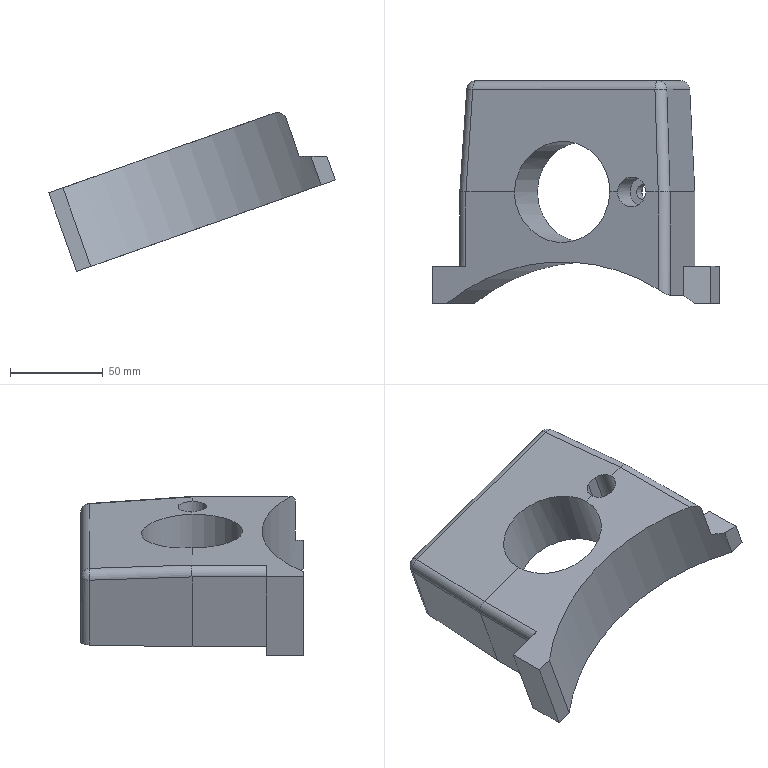Part | STEP file | SLIDE1-1_id622_x_t | 1 solid | 34 faces | box 154.532 x 120 x 85.769 mm | volume 429679 mm3 | plane 19 | cylinder 13 | other 2 | commonest cylinder face diameters 10 x7 8.5 x1 14 x1 16 x1 54.5 x1 71 x1
STEP:
#1=CARTESIAN_POINT('',(40.369,7.5,-42.76));
#2=VERTEX_POINT('',#1);
#3=CARTESIAN_POINT('',(35.121,7.5,-44.618));
#4=VERTEX_POINT('',#3);
#5=CARTESIAN_POINT('',(17.953,7.5,-50.698));
#6=DIRECTION('',(-0.9426,0.,-0.3338));
#7=VECTOR('',#6,1.);
#8=LINE('',#5,#7);
#9=EDGE_CURVE('',#2,#4,#8,.T.);
#10=ORIENTED_EDGE('',*,*,#9,.F.);
#11=CARTESIAN_POINT('',(33.824,7.5,-24.277));
#12=VERTEX_POINT('',#11);
#13=CARTESIAN_POINT('',(33.693,7.5,-23.907));
#14=DIRECTION('',(-0.3338,0.,0.9426));
#15=VECTOR('',#14,1.);
#16=LINE('',#13,#15);
#17=EDGE_CURVE('',#2,#12,#16,.T.);
#18=ORIENTED_EDGE('',*,*,#17,.T.);
#19=CARTESIAN_POINT('',(28.576,7.5,-26.136));
#20=VERTEX_POINT('',#19);
#21=CARTESIAN_POINT('',(-62.86,7.5,-58.515));
#22=DIRECTION('',(-0.9426,0.,-0.3338));
#23=VECTOR('',#22,1.);
#24=LINE('',#21,#23);
#25=EDGE_CURVE('',#12,#20,#24,.T.);
#26=ORIENTED_EDGE('',*,*,#25,.T.);
#27=CARTESIAN_POINT('',(28.444,7.5,-25.765));
#28=DIRECTION('',(0.3338,0.,-0.9426));
#29=VECTOR('',#28,1.);
#30=LINE('',#27,#29);
#31=EDGE_CURVE('',#20,#4,#30,.T.);
#32=ORIENTED_EDGE('',*,*,#31,.T.);
#33=EDGE_LOOP('',(#10,#18,#26,#32));
#34=FACE_OUTER_BOUND('',#33,.T.);
#35=CARTESIAN_POINT('',(33.693,7.5,-23.907));
#36=DIRECTION('',(0.,1.,0.));
#37=DIRECTION('',(0.,0.,1.));
#38=AXIS2_PLACEMENT_3D('',#35,#36,#37);
#39=PLANE('',#38);
#40=ADVANCED_FACE('',(#34),#39,.F.);
#41=CARTESIAN_POINT('',(41.751,0.,-42.27));
#42=VERTEX_POINT('',#41);
#43=CARTESIAN_POINT('',(33.739,0.,-45.108));
#44=VERTEX_POINT('',#43);
#45=CARTESIAN_POINT('',(41.751,0.,-42.27));
#46=CARTESIAN_POINT('',(41.751,-0.5406,-42.27));
#47=CARTESIAN_POINT('',(41.669,-1.031,-42.299));
#48=CARTESIAN_POINT('',(41.271,-2.098,-42.44));
#49=CARTESIAN_POINT('',(40.968,-2.591,-42.547));
#50=CARTESIAN_POINT('',(40.187,-3.42,-42.824));
#51=CARTESIAN_POINT('',(39.693,-3.753,-42.999));
#52=CARTESIAN_POINT('',(38.746,-4.15,-43.334));
#53=CARTESIAN_POINT('',(38.254,-4.25,-43.509));
#54=CARTESIAN_POINT('',(37.236,-4.25,-43.869));
#55=CARTESIAN_POINT('',(36.773,-4.163,-44.033));
#56=CARTESIAN_POINT('',(35.767,-3.74,-44.389));
#57=CARTESIAN_POINT('',(35.303,-3.42,-44.554));
#58=CARTESIAN_POINT('',(34.521,-2.591,-44.83));
#59=CARTESIAN_POINT('',(34.207,-2.066,-44.942));
#60=CARTESIAN_POINT('',(33.832,-1.062,-45.074));
#61=CARTESIAN_POINT('',(33.739,-0.541,-45.108));
#62=CARTESIAN_POINT('',(33.739,0.,-45.108));
#63=B_SPLINE_CURVE_WITH_KNOTS('',3,(#45,#46,#47,#48,#49,#50,#51,#52,#53,#54,#55,#56,#57,#58,#59,#60,#61,#62),.UNSPECIFIED.,.F.,.F.,(4,2,2,2,2,2,2,2,4),(0.,0.125,0.25,0.375,0.5,0.625,0.75,0.875,1.),.UNSPECIFIED.);
#64=EDGE_CURVE('',#42,#44,#63,.T.);
#65=ORIENTED_EDGE('',*,*,#64,.T.);
#66=CARTESIAN_POINT('',(33.739,0.,-45.108));
#67=CARTESIAN_POINT('',(33.739,0.5406,-45.108));
#68=CARTESIAN_POINT('',(33.821,1.031,-45.079));
#69=CARTESIAN_POINT('',(34.219,2.098,-44.938));
#70=CARTESIAN_POINT('',(34.521,2.591,-44.83));
#71=CARTESIAN_POINT('',(35.303,3.42,-44.554));
#72=CARTESIAN_POINT('',(35.797,3.753,-44.379));
#73=CARTESIAN_POINT('',(36.743,4.15,-44.044));
#74=CARTESIAN_POINT('',(37.236,4.25,-43.869));
#75=CARTESIAN_POINT('',(38.254,4.25,-43.509));
#76=CARTESIAN_POINT('',(38.717,4.163,-43.345));
#77=CARTESIAN_POINT('',(39.722,3.74,-42.989));
#78=CARTESIAN_POINT('',(40.187,3.42,-42.824));
#79=CARTESIAN_POINT('',(40.968,2.591,-42.547));
#80=CARTESIAN_POINT('',(41.282,2.066,-42.436));
#81=CARTESIAN_POINT('',(41.657,1.062,-42.304));
#82=CARTESIAN_POINT('',(41.751,0.541,-42.27));
#83=CARTESIAN_POINT('',(41.751,0.,-42.27));
#84=B_SPLINE_CURVE_WITH_KNOTS('',3,(#66,#67,#68,#69,#70,#71,#72,#73,#74,#75,#76,#77,#78,#79,#80,#81,#82,#83),.UNSPECIFIED.,.F.,.F.,(4,2,2,2,2,2,2,2,4),(0.,0.125,0.25,0.375,0.5,0.625,0.75,0.875,1.),.UNSPECIFIED.);
#85=EDGE_CURVE('',#44,#42,#84,.T.);
#86=ORIENTED_EDGE('',*,*,#85,.T.);
#87=EDGE_LOOP('',(#65,#86));
#88=FACE_BOUND('',#87,.T.);
#89=ORIENTED_EDGE('',*,*,#9,.T.);
#90=CARTESIAN_POINT('',(35.121,7.5,-44.618));
#91=CARTESIAN_POINT('',(34.318,7.184,-44.903));
#92=CARTESIAN_POINT('',(33.619,6.764,-45.15));
#93=CARTESIAN_POINT('',(32.238,5.548,-45.639));
#94=CARTESIAN_POINT('',(31.648,4.807,-45.848));
#95=CARTESIAN_POINT('',(30.744,3.127,-46.168));
#96=CARTESIAN_POINT('',(30.438,2.182,-46.276));
#97=CARTESIAN_POINT('',(30.161,0.3618,-46.374));
#98=CARTESIAN_POINT('',(30.176,-0.5477,-46.369));
#99=CARTESIAN_POINT('',(30.469,-2.281,-46.265));
#100=CARTESIAN_POINT('',(30.74,-3.113,-46.169));
#101=CARTESIAN_POINT('',(31.624,-4.769,-45.856));
#102=CARTESIAN_POINT('',(32.207,-5.516,-45.65));
#103=CARTESIAN_POINT('',(33.606,-6.757,-45.155));
#104=CARTESIAN_POINT('',(34.429,-7.244,-44.863));
#105=CARTESIAN_POINT('',(36.069,-7.854,-44.283));
#106=CARTESIAN_POINT('',(36.915,-8.,-43.983));
#107=CARTESIAN_POINT('',(38.575,-8.,-43.395));
#108=CARTESIAN_POINT('',(39.394,-7.864,-43.105));
#109=CARTESIAN_POINT('',(41.088,-7.234,-42.505));
#110=CARTESIAN_POINT('',(41.883,-6.757,-42.223));
#111=CARTESIAN_POINT('',(43.283,-5.516,-41.728));
#112=CARTESIAN_POINT('',(43.879,-4.743,-41.517));
#113=CARTESIAN_POINT('',(44.736,-3.139,-41.213));
#114=CARTESIAN_POINT('',(45.02,-2.281,-41.113));
#115=CARTESIAN_POINT('',(45.314,-0.5477,-41.009));
#116=CARTESIAN_POINT('',(45.333,0.3322,-41.002));
#117=CARTESIAN_POINT('',(45.047,2.212,-41.103));
#118=CARTESIAN_POINT('',(44.746,3.127,-41.21));
#119=CARTESIAN_POINT('',(43.841,4.807,-41.53));
#120=CARTESIAN_POINT('',(43.22,5.576,-41.75));
#121=CARTESIAN_POINT('',(41.903,6.736,-42.216));
#122=CARTESIAN_POINT('',(41.172,7.184,-42.475));
#123=CARTESIAN_POINT('',(40.369,7.5,-42.76));
#124=B_SPLINE_CURVE_WITH_KNOTS('',3,(#90,#91,#92,#93,#94,#95,#96,#97,#98,#99,#100,#101,#102,#103,#104,#105,#106,#107,#108,#109,#110,#111,#112,#113,#114,#115,#116,#117,#118,#119,#120,#121,#122,#123),.UNSPECIFIED.,.F.,.F.,(4,2,2,2,2,2,2,2,2,2,2,2,2,2,2,2,4),(0.,0.0625,0.125,0.1875,0.25,0.3125,0.375,0.4375,0.5,0.5625,0.625,0.6875,0.75,0.8125,0.875,0.9375,1.),.UNSPECIFIED.);
#125=EDGE_CURVE('',#4,#2,#124,.T.);
#126=ORIENTED_EDGE('',*,*,#125,.T.);
#127=EDGE_LOOP('',(#89,#126));
#128=FACE_BOUND('',#127,.T.);
#129=CARTESIAN_POINT('',(17.953,60.,-50.698));
#130=DIRECTION('',(-0.3338,0.,0.9426));
#131=DIRECTION('',(0.9426,0.,0.3338));
#132=AXIS2_PLACEMENT_3D('',#129,#130,#131);
#133=PLANE('',#132);
#134=ADVANCED_FACE('',(#88,#128),#133,.T.);
#135=CARTESIAN_POINT('',(38.61,0.,-22.166));
#136=VERTEX_POINT('',#135);
#137=CARTESIAN_POINT('',(38.61,0.,-22.166));
#138=CARTESIAN_POINT('',(38.647,2.147,-22.272));
#139=CARTESIAN_POINT('',(37.913,3.669,-22.616));
#140=CARTESIAN_POINT('',(37.304,4.623,-22.885));
#141=CARTESIAN_POINT('',(37.224,4.745,-22.92));
#142=CARTESIAN_POINT('',(37.104,4.917,-22.972));
#143=CARTESIAN_POINT('',(37.042,5.002,-22.999));
#144=CARTESIAN_POINT('',(36.854,5.25,-23.079));
#145=CARTESIAN_POINT('',(36.723,5.409,-23.134));
#146=CARTESIAN_POINT('',(36.317,5.863,-23.303));
#147=CARTESIAN_POINT('',(36.028,6.137,-23.421));
#148=CARTESIAN_POINT('',(35.127,6.87,-23.781));
#149=CARTESIAN_POINT('',(34.479,7.24,-24.031));
#150=CARTESIAN_POINT('',(33.824,7.5,-24.277));
#151=B_SPLINE_CURVE_WITH_KNOTS('',3,(#137,#138,#139,#140,#141,#142,#143,#144,#145,#146,#147,#148,#149,#150),.UNSPECIFIED.,.F.,.F.,(4,2,2,2,2,2,4),(0.,0.5,0.5313,0.5625,0.625,0.75,1.),.UNSPECIFIED.);
#152=EDGE_CURVE('',#136,#12,#151,.T.);
#153=ORIENTED_EDGE('',*,*,#152,.T.);
#154=ORIENTED_EDGE('',*,*,#17,.F.);
#155=ORIENTED_EDGE('',*,*,#125,.F.);
#156=ORIENTED_EDGE('',*,*,#31,.F.);
#157=CARTESIAN_POINT('',(23.528,0.,-27.507));
#158=VERTEX_POINT('',#157);
#159=CARTESIAN_POINT('',(28.576,7.5,-26.136));
#160=CARTESIAN_POINT('',(27.247,6.981,-26.577));
#161=CARTESIAN_POINT('',(25.923,6.003,-26.992));
#162=CARTESIAN_POINT('',(24.896,4.477,-27.271));
#163=CARTESIAN_POINT('',(24.881,4.452,-27.275));
#164=CARTESIAN_POINT('',(24.804,4.331,-27.295));
#165=CARTESIAN_POINT('',(24.765,4.268,-27.306));
#166=CARTESIAN_POINT('',(24.648,4.073,-27.336));
#167=CARTESIAN_POINT('',(24.569,3.933,-27.356));
#168=CARTESIAN_POINT('',(24.334,3.485,-27.414));
#169=CARTESIAN_POINT('',(24.18,3.147,-27.45));
#170=CARTESIAN_POINT('',(23.764,2.007,-27.534));
#171=CARTESIAN_POINT('',(23.546,1.073,-27.56));
#172=CARTESIAN_POINT('',(23.528,0.,-27.507));
#173=B_SPLINE_CURVE_WITH_KNOTS('',3,(#159,#160,#161,#162,#163,#164,#165,#166,#167,#168,#169,#170,#171,#172),.UNSPECIFIED.,.F.,.F.,(4,2,2,2,2,2,4),(0.,0.5,0.5312,0.5625,0.625,0.75,1.),.UNSPECIFIED.);
#174=EDGE_CURVE('',#20,#158,#173,.T.);
#175=ORIENTED_EDGE('',*,*,#174,.T.);
#176=CARTESIAN_POINT('',(38.61,0.,-22.166));
#177=CARTESIAN_POINT('',(38.61,-0.979,-22.166));
#178=CARTESIAN_POINT('',(38.455,-1.94,-22.22));
#179=CARTESIAN_POINT('',(37.705,-3.95,-22.486));
#180=CARTESIAN_POINT('',(37.137,-4.876,-22.687));
#181=CARTESIAN_POINT('',(35.665,-6.437,-23.208));
#182=CARTESIAN_POINT('',(34.753,-7.056,-23.531));
#183=CARTESIAN_POINT('',(32.936,-7.82,-24.175));
#184=CARTESIAN_POINT('',(31.99,-8.,-24.51));
#185=CARTESIAN_POINT('',(30.147,-8.,-25.163));
#186=CARTESIAN_POINT('',(29.24,-7.836,-25.484));
#187=CARTESIAN_POINT('',(27.346,-7.041,-26.155));
#188=CARTESIAN_POINT('',(26.472,-6.437,-26.464));
#189=CARTESIAN_POINT('',(25.,-4.876,-26.985));
#190=CARTESIAN_POINT('',(24.417,-3.909,-27.192));
#191=CARTESIAN_POINT('',(23.697,-1.98,-27.447));
#192=CARTESIAN_POINT('',(23.528,-0.9797,-27.507));
#193=CARTESIAN_POINT('',(23.528,0.,-27.507));
#194=B_SPLINE_CURVE_WITH_KNOTS('',3,(#176,#177,#178,#179,#180,#181,#182,#183,#184,#185,#186,#187,#188,#189,#190,#191,#192,#193),.UNSPECIFIED.,.F.,.F.,(4,2,2,2,2,2,2,2,4),(0.,0.125,0.25,0.375,0.5,0.625,0.75,0.875,1.),.UNSPECIFIED.);
#195=EDGE_CURVE('',#136,#158,#194,.T.);
#196=ORIENTED_EDGE('',*,*,#195,.F.);
#197=EDGE_LOOP('',(#153,#154,#155,#156,#175,#196));
#198=FACE_OUTER_BOUND('',#197,.T.);
#199=CARTESIAN_POINT('',(31.069,0.,-24.836));
#200=DIRECTION('',(-0.3338,0.,0.9426));
#201=DIRECTION('',(0.9426,0.,0.3338));
#202=AXIS2_PLACEMENT_3D('',#199,#200,#201);
#203=CYLINDRICAL_SURFACE('',#202,8.);
#204=ADVANCED_FACE('',(#198),#203,.F.);
#205=CARTESIAN_POINT('',(-32.119,0.,-47.212));
#206=VERTEX_POINT('',#205);
#207=CARTESIAN_POINT('',(19.255,0.,-29.02));
#208=VERTEX_POINT('',#207);
#209=CARTESIAN_POINT('',(-32.119,0.,-47.212));
#210=CARTESIAN_POINT('',(-32.09,1.66,-47.294));
#211=CARTESIAN_POINT('',(-31.917,3.315,-47.325));
#212=CARTESIAN_POINT('',(-31.443,5.788,-47.295));
#213=CARTESIAN_POINT('',(-31.228,6.699,-47.269));
#214=CARTESIAN_POINT('',(-30.741,8.388,-47.19));
#215=CARTESIAN_POINT('',(-30.459,9.217,-47.137));
#216=CARTESIAN_POINT('',(-29.821,10.844,-47.001));
#217=CARTESIAN_POINT('',(-29.436,11.707,-46.913));
#218=CARTESIAN_POINT('',(-28.61,13.332,-46.711));
#219=CARTESIAN_POINT('',(-28.156,14.128,-46.594));
#220=CARTESIAN_POINT('',(-26.675,16.465,-46.2));
#221=CARTESIAN_POINT('',(-25.52,17.952,-45.873));
#222=CARTESIAN_POINT('',(-22.997,20.586,-45.126));
#223=CARTESIAN_POINT('',(-21.583,21.785,-44.692));
#224=CARTESIAN_POINT('',(-18.596,23.831,-43.748));
#225=CARTESIAN_POINT('',(-17.069,24.659,-43.253));
#226=CARTESIAN_POINT('',(-14.632,25.676,-42.447));
#227=CARTESIAN_POINT('',(-13.874,25.946,-42.194));
#228=CARTESIAN_POINT('',(-12.272,26.432,-41.653));
#229=CARTESIAN_POINT('',(-11.46,26.634,-41.377));
#230=CARTESIAN_POINT('',(-9.815,26.956,-40.812));
#231=CARTESIAN_POINT('',(-9.084,27.06,-40.559));
#232=CARTESIAN_POINT('',(-7.523,27.212,-40.015));
#233=CARTESIAN_POINT('',(-6.741,27.25,-39.74));
#234=CARTESIAN_POINT('',(-4.385,27.25,-38.906));
#235=CARTESIAN_POINT('',(-2.829,27.098,-38.347));
#236=CARTESIAN_POINT('',(-0.5194,26.643,-37.503));
#237=CARTESIAN_POINT('',(0.3325,26.432,-37.19));
#238=CARTESIAN_POINT('',(1.918,25.946,-36.602));
#239=CARTESIAN_POINT('',(2.698,25.662,-36.309));
#240=CARTESIAN_POINT('',(4.234,25.012,-35.729));
#241=CARTESIAN_POINT('',(5.047,24.617,-35.419));
#242=CARTESIAN_POINT('',(6.566,23.775,-34.835));
#243=CARTESIAN_POINT('',(7.305,23.312,-34.547));
#244=CARTESIAN_POINT('',(9.459,21.8,-33.7));
#245=CARTESIAN_POINT('',(10.847,20.593,-33.142));
#246=CARTESIAN_POINT('',(14.512,16.62,-31.623));
#247=CARTESIAN_POINT('',(16.417,13.416,-30.77));
#248=CARTESIAN_POINT('',(17.929,9.184,-30.));
#249=CARTESIAN_POINT('',(18.17,8.387,-29.87));
#250=CARTESIAN_POINT('',(18.598,6.698,-29.625));
#251=CARTESIAN_POINT('',(18.773,5.839,-29.515));
#252=CARTESIAN_POINT('',(19.048,4.089,-29.32));
#253=CARTESIAN_POINT('',(19.133,3.313,-29.247));
#254=CARTESIAN_POINT('',(19.248,1.658,-29.114));
#255=CARTESIAN_POINT('',(19.269,0.8298,-29.061));
#256=CARTESIAN_POINT('',(19.255,0.,-29.02));
#257=B_SPLINE_CURVE_WITH_KNOTS('',3,(#209,#210,#211,#212,#213,#214,#215,#216,#217,#218,#219,#220,#221,#222,#223,#224,#225,#226,#227,#228,#229,#230,#231,#232,#233,#234,#235,#236,#237,#238,#239,#240,#241,#242,#243,#244,#245,#246,#247,#248,#249,#250,#251,#252,#253,#254,#255,#256),.UNSPECIFIED.,.F.,.F.,(4,2,2,2,2,2,2,2,2,2,2,2,2,2,2,2,2,2,2,2,2,2,2,4),(0.,0.0625,0.09375,0.125,0.1562,0.1875,0.25,0.3125,0.375,0.4062,0.4375,0.4687,0.5,0.5625,0.5937,0.625,0.6562,0.6875,0.75,0.875,0.9062,0.9375,0.9688,1.),.UNSPECIFIED.);
#258=EDGE_CURVE('',#206,#208,#257,.T.);
#259=ORIENTED_EDGE('',*,*,#258,.T.);
#260=CARTESIAN_POINT('',(50.126,0.,-18.087));
#261=DIRECTION('',(-0.9426,0.,-0.3338));
#262=VECTOR('',#261,1.);
#263=LINE('',#260,#262);
#264=EDGE_CURVE('',#158,#208,#263,.T.);
#265=ORIENTED_EDGE('',*,*,#264,.F.);
#266=ORIENTED_EDGE('',*,*,#174,.F.);
#267=ORIENTED_EDGE('',*,*,#25,.F.);
#268=ORIENTED_EDGE('',*,*,#152,.F.);
#269=CARTESIAN_POINT('',(45.416,-0.000000024,-19.755));
#270=VERTEX_POINT('',#269);
#271=CARTESIAN_POINT('',(50.126,0.,-18.087));
#272=DIRECTION('',(-0.9426,0.,-0.3338));
#273=VECTOR('',#272,1.);
#274=LINE('',#271,#273);
#275=EDGE_CURVE('',#270,#136,#274,.T.);
#276=ORIENTED_EDGE('',*,*,#275,.F.);
#277=CARTESIAN_POINT('',(43.656,55.262,-23.451));
#278=VERTEX_POINT('',#277);
#279=CARTESIAN_POINT('',(43.656,55.262,-23.451));
#280=CARTESIAN_POINT('',(44.243,36.841,-22.219));
#281=CARTESIAN_POINT('',(44.83,18.421,-20.987));
#282=CARTESIAN_POINT('',(45.416,-0.000000061,-19.755));
#283=B_SPLINE_CURVE_WITH_KNOTS('',3,(#279,#280,#281,#282),.UNSPECIFIED.,.F.,.F.,(4,4),(0.,1.),.UNSPECIFIED.);
#284=EDGE_CURVE('',#278,#270,#283,.T.);
#285=ORIENTED_EDGE('',*,*,#284,.F.);
#286=CARTESIAN_POINT('',(-54.587,55.262,-58.241));
#287=VERTEX_POINT('',#286);
#288=CARTESIAN_POINT('',(-61.119,55.262,-60.554));
#289=DIRECTION('',(0.9426,0.,0.3338));
#290=VECTOR('',#289,1.);
#291=LINE('',#288,#290);
#292=EDGE_CURVE('',#287,#278,#291,.T.);
#293=ORIENTED_EDGE('',*,*,#292,.F.);
#294=CARTESIAN_POINT('',(-58.281,-0.000000024,-56.476));
#295=VERTEX_POINT('',#294);
#296=CARTESIAN_POINT('',(-58.281,-0.000000061,-56.476));
#297=CARTESIAN_POINT('',(-57.05,18.421,-57.065));
#298=CARTESIAN_POINT('',(-55.818,36.841,-57.653));
#299=CARTESIAN_POINT('',(-54.587,55.262,-58.241));
#300=B_SPLINE_CURVE_WITH_KNOTS('',3,(#296,#297,#298,#299),.UNSPECIFIED.,.F.,.F.,(4,4),(0.,1.),.UNSPECIFIED.);
#301=EDGE_CURVE('',#295,#287,#300,.T.);
#302=ORIENTED_EDGE('',*,*,#301,.F.);
#303=CARTESIAN_POINT('',(50.126,0.,-18.087));
#304=DIRECTION('',(-0.9426,0.,-0.3338));
#305=VECTOR('',#304,1.);
#306=LINE('',#303,#305);
#307=EDGE_CURVE('',#206,#295,#306,.T.);
#308=ORIENTED_EDGE('',*,*,#307,.F.);
#309=EDGE_LOOP('',(#259,#265,#266,#267,#268,#276,#285,#293,#302,#308));
#310=FACE_OUTER_BOUND('',#309,.T.);
#311=CARTESIAN_POINT('',(-61.941,60.,-61.108));
#312=DIRECTION('',(0.3333,-0.05234,-0.9413));
#313=DIRECTION('',(-0.9426,0.,-0.3338));
#314=AXIS2_PLACEMENT_3D('',#311,#312,#313);
#315=PLANE('',#314);
#316=ADVANCED_FACE('',(#310),#315,.F.);
#317=CARTESIAN_POINT('',(31.606,0.,-63.897));
#318=VERTEX_POINT('',#317);
#319=CARTESIAN_POINT('',(5.919,0.,-72.994));
#320=DIRECTION('',(-0.3338,0.,0.9426));
#321=DIRECTION('',(0.9426,0.,0.3338));
#322=AXIS2_PLACEMENT_3D('',#319,#320,#321);
#323=CIRCLE('',#322,27.25);
#324=EDGE_CURVE('',#318,#318,#323,.T.);
#325=ORIENTED_EDGE('',*,*,#324,.F.);
#326=EDGE_LOOP('',(#325));
#327=FACE_BOUND('',#326,.T.);
#328=CARTESIAN_POINT('',(19.255,0.,-29.02));
#329=CARTESIAN_POINT('',(19.255,-0.8335,-29.02));
#330=CARTESIAN_POINT('',(19.219,-1.663,-29.032));
#331=CARTESIAN_POINT('',(19.076,-3.316,-29.083));
#332=CARTESIAN_POINT('',(18.977,-4.09,-29.118));
#333=CARTESIAN_POINT('',(18.674,-5.827,-29.225));
#334=CARTESIAN_POINT('',(18.484,-6.684,-29.293));
#335=CARTESIAN_POINT('',(18.026,-8.375,-29.455));
#336=CARTESIAN_POINT('',(17.771,-9.175,-29.545));
#337=CARTESIAN_POINT('',(16.812,-11.743,-29.885));
#338=CARTESIAN_POINT('',(16.038,-13.337,-30.159));
#339=CARTESIAN_POINT('',(14.097,-16.486,-30.846));
#340=CARTESIAN_POINT('',(12.985,-17.939,-31.24));
#341=CARTESIAN_POINT('',(10.478,-20.599,-32.128));
#342=CARTESIAN_POINT('',(9.077,-21.8,-32.624));
#343=CARTESIAN_POINT('',(6.898,-23.312,-33.396));
#344=CARTESIAN_POINT('',(6.151,-23.775,-33.66));
#345=CARTESIAN_POINT('',(4.617,-24.617,-34.203));
#346=CARTESIAN_POINT('',(3.797,-25.011,-34.493));
#347=CARTESIAN_POINT('',(2.249,-25.662,-35.042));
#348=CARTESIAN_POINT('',(1.463,-25.946,-35.32));
#349=CARTESIAN_POINT('',(-0.1308,-26.432,-35.884));
#350=CARTESIAN_POINT('',(-0.9859,-26.643,-36.187));
#351=CARTESIAN_POINT('',(-3.303,-27.098,-37.008));
#352=CARTESIAN_POINT('',(-4.861,-27.25,-37.56));
#353=CARTESIAN_POINT('',(-7.218,-27.25,-38.394));
#354=CARTESIAN_POINT('',(-8.,-27.212,-38.671));
#355=CARTESIAN_POINT('',(-9.558,-27.06,-39.223));
#356=CARTESIAN_POINT('',(-10.287,-26.956,-39.481));
#357=CARTESIAN_POINT('',(-11.925,-26.634,-40.061));
#358=CARTESIAN_POINT('',(-12.733,-26.432,-40.347));
#359=CARTESIAN_POINT('',(-14.327,-25.946,-40.912));
#360=CARTESIAN_POINT('',(-15.081,-25.676,-41.178));
#361=CARTESIAN_POINT('',(-17.501,-24.659,-42.036));
#362=CARTESIAN_POINT('',(-19.004,-23.837,-42.568));
#363=CARTESIAN_POINT('',(-21.972,-21.779,-43.619));
#364=CARTESIAN_POINT('',(-23.342,-20.599,-44.104));
#365=CARTESIAN_POINT('',(-25.849,-17.939,-44.992));
#366=CARTESIAN_POINT('',(-26.982,-16.453,-45.393));
#367=CARTESIAN_POINT('',(-28.407,-14.141,-45.898));
#368=CARTESIAN_POINT('',(-28.843,-13.349,-46.052));
#369=CARTESIAN_POINT('',(-29.638,-11.722,-46.333));
#370=CARTESIAN_POINT('',(-30.009,-10.852,-46.465));
#371=CARTESIAN_POINT('',(-30.622,-9.209,-46.682));
#372=CARTESIAN_POINT('',(-30.89,-8.376,-46.777));
#373=CARTESIAN_POINT('',(-31.348,-6.685,-46.939));
#374=CARTESIAN_POINT('',(-31.547,-5.778,-47.01));
#375=CARTESIAN_POINT('',(-31.976,-3.32,-47.161));
#376=CARTESIAN_POINT('',(-32.119,-1.667,-47.212));
#377=CARTESIAN_POINT('',(-32.119,0.,-47.212));
#378=B_SPLINE_CURVE_WITH_KNOTS('',3,(#328,#329,#330,#331,#332,#333,#334,#335,#336,#337,#338,#339,#340,#341,#342,#343,#344,#345,#346,#347,#348,#349,#350,#351,#352,#353,#354,#355,#356,#357,#358,#359,#360,#361,#362,#363,#364,#365,#366,#367,#368,#369,#370,#371,#372,#373,#374,#375,#376,#377),.UNSPECIFIED.,.F.,.F.,(4,2,2,2,2,2,2,2,2,2,2,2,2,2,2,2,2,2,2,2,2,2,2,2,4),(0.,0.03125,0.0625,0.09375,0.125,0.1875,0.25,0.3125,0.3438,0.375,0.4062,0.4375,0.5,0.5312,0.5625,0.5938,0.625,0.6875,0.75,0.8125,0.8438,0.875,0.9062,0.9375,1.),.UNSPECIFIED.);
#379=EDGE_CURVE('',#208,#206,#378,.T.);
#380=ORIENTED_EDGE('',*,*,#379,.F.);
#381=ORIENTED_EDGE('',*,*,#258,.F.);
#382=EDGE_LOOP('',(#380,#381));
#383=FACE_BOUND('',#382,.T.);
#384=CARTESIAN_POINT('',(-6.432,0.,-38.116));
#385=DIRECTION('',(-0.3338,0.,0.9426));
#386=DIRECTION('',(0.9426,0.,0.3338));
#387=AXIS2_PLACEMENT_3D('',#384,#385,#386);
#388=CYLINDRICAL_SURFACE('',#387,27.25);
#389=ADVANCED_FACE('',(#327,#383),#388,.F.);
#390=ORIENTED_EDGE('',*,*,#85,.F.);
#391=ORIENTED_EDGE('',*,*,#64,.F.);
#392=EDGE_LOOP('',(#390,#391));
#393=FACE_BOUND('',#392,.T.);
#394=CARTESIAN_POINT('',(36.409,0.,-52.649));
#395=VERTEX_POINT('',#394);
#396=CARTESIAN_POINT('',(40.415,0.,-51.23));
#397=DIRECTION('',(-0.3338,0.,0.9426));
#398=DIRECTION('',(-0.9426,0.,-0.3338));
#399=AXIS2_PLACEMENT_3D('',#396,#397,#398);
#400=CIRCLE('',#399,4.25);
#401=EDGE_CURVE('',#395,#395,#400,.T.);
#402=ORIENTED_EDGE('',*,*,#401,.F.);
#403=EDGE_LOOP('',(#402));
#404=FACE_BOUND('',#403,.T.);
#405=CARTESIAN_POINT('',(46.09,0.,-67.255));
#406=DIRECTION('',(0.3338,0.,-0.9426));
#407=DIRECTION('',(-0.9426,0.,-0.3338));
#408=AXIS2_PLACEMENT_3D('',#405,#406,#407);
#409=CYLINDRICAL_SURFACE('',#408,4.25);
#410=ADVANCED_FACE('',(#393,#404),#409,.F.);
#411=CARTESIAN_POINT('',(50.03,55.262,-26.491));
#412=VERTEX_POINT('',#411);
#413=CARTESIAN_POINT('',(51.794,-0.000000012,-22.797));
#414=VERTEX_POINT('',#413);
#415=CARTESIAN_POINT('',(50.03,55.262,-26.491));
#416=DIRECTION('',(0.03184,-0.9973,0.06665));
#417=VECTOR('',#416,1.);
#418=LINE('',#415,#417);
#419=EDGE_CURVE('',#412,#414,#418,.T.);
#420=ORIENTED_EDGE('',*,*,#419,.F.);
#421=CARTESIAN_POINT('',(45.323,55.,-28.158));
#422=DIRECTION('',(-0.03182,0.9973,-0.06671));
#423=DIRECTION('',(0.,0.06675,0.9978));
#424=AXIS2_PLACEMENT_3D('',#421,#422,#423);
#425=CIRCLE('',#424,5.);
#426=EDGE_CURVE('',#278,#412,#425,.T.);
#427=ORIENTED_EDGE('',*,*,#426,.F.);
#428=ORIENTED_EDGE('',*,*,#284,.T.);
#429=CARTESIAN_POINT('',(51.794,0.,-22.797));
#430=CARTESIAN_POINT('',(51.76,0.000000654,-22.7));
#431=CARTESIAN_POINT('',(51.712,0.00167,-22.576));
#432=CARTESIAN_POINT('',(51.579,0.008348,-22.278));
#433=CARTESIAN_POINT('',(51.467,0.01493,-22.06));
#434=CARTESIAN_POINT('',(51.206,0.03024,-21.622));
#435=CARTESIAN_POINT('',(51.02,0.03714,-21.372));
#436=CARTESIAN_POINT('',(50.58,0.04562,-20.882));
#437=CARTESIAN_POINT('',(50.337,0.0488,-20.66));
#438=CARTESIAN_POINT('',(49.811,0.05305,-20.267));
#439=CARTESIAN_POINT('',(49.479,0.05411,-20.073));
#440=CARTESIAN_POINT('',(48.99,0.05411,-19.84));
#441=CARTESIAN_POINT('',(48.69,0.05285,-19.72));
#442=CARTESIAN_POINT('',(47.967,0.04781,-19.535));
#443=CARTESIAN_POINT('',(47.541,0.04399,-19.484));
#444=CARTESIAN_POINT('',(47.006,0.03686,-19.463));
#445=CARTESIAN_POINT('',(46.78,0.03199,-19.464));
#446=CARTESIAN_POINT('',(46.008,0.009667,-19.571));
#447=CARTESIAN_POINT('',(45.638,0.000001488,-19.677));
#448=CARTESIAN_POINT('',(45.416,0.,-19.755));
#449=B_SPLINE_CURVE_WITH_KNOTS('',3,(#429,#430,#431,#432,#433,#434,#435,#436,#437,#438,#439,#440,#441,#442,#443,#444,#445,#446,#447,#448),.UNSPECIFIED.,.F.,.F.,(4,2,2,2,2,2,2,2,2,4),(0.,0.0625,0.125,0.25,0.375,0.5,0.625,0.75,0.875,1.),.UNSPECIFIED.);
#450=EDGE_CURVE('',#414,#270,#449,.T.);
#451=ORIENTED_EDGE('',*,*,#450,.F.);
#452=EDGE_LOOP('',(#420,#427,#428,#451));
#453=FACE_OUTER_BOUND('',#452,.T.);
#454=CARTESIAN_POINT('',(47.095,-0.5481,-24.442));
#455=DIRECTION('',(-0.03182,0.9973,-0.06671));
#456=DIRECTION('',(0.,0.06675,0.9978));
#457=AXIS2_PLACEMENT_3D('',#454,#455,#456);
#458=CYLINDRICAL_SURFACE('',#457,5.);
#459=ADVANCED_FACE('',(#453),#458,.T.);
#460=CARTESIAN_POINT('',(45.413,-52.673,-19.757));
#461=VERTEX_POINT('',#460);
#462=CARTESIAN_POINT('',(45.413,-52.673,-19.757));
#463=DIRECTION('',(0.00006131,1.,0.00002171));
#464=VECTOR('',#463,1.);
#465=LINE('',#462,#464);
#466=EDGE_CURVE('',#461,#270,#465,.T.);
#467=ORIENTED_EDGE('',*,*,#466,.F.);
#468=CARTESIAN_POINT('',(51.795,-55.8,-22.801));
#469=VERTEX_POINT('',#468);
#470=CARTESIAN_POINT('',(45.413,-52.673,-19.757));
#471=CARTESIAN_POINT('',(46.583,-53.403,-19.342));
#472=CARTESIAN_POINT('',(47.867,-54.147,-19.367));
#473=CARTESIAN_POINT('',(50.235,-55.356,-20.381));
#474=CARTESIAN_POINT('',(51.312,-55.8,-21.436));
#475=CARTESIAN_POINT('',(51.795,-55.8,-22.801));
#476=B_SPLINE_CURVE_WITH_KNOTS('',3,(#470,#471,#472,#473,#474,#475),.UNSPECIFIED.,.F.,.F.,(4,2,4),(0.,0.5,1.),.UNSPECIFIED.);
#477=EDGE_CURVE('',#461,#469,#476,.T.);
#478=ORIENTED_EDGE('',*,*,#477,.T.);
#479=CARTESIAN_POINT('',(51.794,0.,-22.797));
#480=DIRECTION('',(0.0000205,-1.,-0.00005788));
#481=VECTOR('',#480,1.);
#482=LINE('',#479,#481);
#483=EDGE_CURVE('',#414,#469,#482,.T.);
#484=ORIENTED_EDGE('',*,*,#483,.F.);
#485=ORIENTED_EDGE('',*,*,#450,.T.);
#486=EDGE_LOOP('',(#467,#478,#484,#485));
#487=FACE_OUTER_BOUND('',#486,.T.);
#488=CARTESIAN_POINT('',(47.082,-60.304,-24.47));
#489=DIRECTION('',(0.,1.,0.));
#490=DIRECTION('',(0.,0.,1.));
#491=AXIS2_PLACEMENT_3D('',#488,#489,#490);
#492=CYLINDRICAL_SURFACE('',#491,5.);
#493=ADVANCED_FACE('',(#487),#492,.T.);
#494=CARTESIAN_POINT('',(58.948,-55.8,-43.));
#495=VERTEX_POINT('',#494);
#496=CARTESIAN_POINT('',(58.948,-40.,-43.));
#497=VERTEX_POINT('',#496);
#498=CARTESIAN_POINT('',(58.948,60.,-43.));
#499=DIRECTION('',(0.,1.,0.));
#500=VECTOR('',#499,1.);
#501=LINE('',#498,#500);
#502=EDGE_CURVE('',#495,#497,#501,.T.);
#503=ORIENTED_EDGE('',*,*,#502,.F.);
#504=CARTESIAN_POINT('',(65.199,-60.,-43.));
#505=VERTEX_POINT('',#504);
#506=CARTESIAN_POINT('',(-4.703,-146.2,-43.));
#507=DIRECTION('',(0.,0.,-1.));
#508=DIRECTION('',(-1.,0.,0.));
#509=AXIS2_PLACEMENT_3D('',#506,#507,#508);
#510=ELLIPSE('',#509,115.102,108.5);
#511=EDGE_CURVE('',#495,#505,#510,.T.);
#512=ORIENTED_EDGE('',*,*,#511,.T.);
#513=CARTESIAN_POINT('',(73.8,-60.,-43.));
#514=VERTEX_POINT('',#513);
#515=CARTESIAN_POINT('',(0.,-60.,-43.));
#516=DIRECTION('',(-1.,0.,0.));
#517=VECTOR('',#516,1.);
#518=LINE('',#515,#517);
#519=EDGE_CURVE('',#514,#505,#518,.T.);
#520=ORIENTED_EDGE('',*,*,#519,.F.);
#521=CARTESIAN_POINT('',(73.8,-40.,-43.));
#522=VERTEX_POINT('',#521);
#523=CARTESIAN_POINT('',(73.8,-60.,-43.));
#524=DIRECTION('',(0.,-1.,0.));
#525=VECTOR('',#524,1.);
#526=LINE('',#523,#525);
#527=EDGE_CURVE('',#522,#514,#526,.T.);
#528=ORIENTED_EDGE('',*,*,#527,.F.);
#529=CARTESIAN_POINT('',(0.,-40.,-43.));
#530=DIRECTION('',(1.,0.,0.));
#531=VECTOR('',#530,1.);
#532=LINE('',#529,#531);
#533=EDGE_CURVE('',#497,#522,#532,.T.);
#534=ORIENTED_EDGE('',*,*,#533,.F.);
#535=EDGE_LOOP('',(#503,#512,#520,#528,#534));
#536=FACE_OUTER_BOUND('',#535,.T.);
#537=CARTESIAN_POINT('',(58.948,-60.,-43.));
#538=DIRECTION('',(0.,0.,1.));
#539=DIRECTION('',(1.,0.,0.));
#540=AXIS2_PLACEMENT_3D('',#537,#538,#539);
#541=PLANE('',#540);
#542=ADVANCED_FACE('',(#536),#541,.T.);
#543=ORIENTED_EDGE('',*,*,#307,.T.);
#544=CARTESIAN_POINT('',(-58.278,-40.,-56.475));
#545=VERTEX_POINT('',#544);
#546=CARTESIAN_POINT('',(-58.278,-40.,-56.475));
#547=CARTESIAN_POINT('',(-58.279,-26.667,-56.476));
#548=CARTESIAN_POINT('',(-58.28,-13.333,-56.476));
#549=CARTESIAN_POINT('',(-58.281,0.,-56.476));
#550=B_SPLINE_CURVE_WITH_KNOTS('',3,(#546,#547,#548,#549),.UNSPECIFIED.,.F.,.F.,(4,4),(0.,1.),.UNSPECIFIED.);
#551=EDGE_CURVE('',#545,#295,#550,.T.);
#552=ORIENTED_EDGE('',*,*,#551,.F.);
#553=CARTESIAN_POINT('',(-76.188,-40.,-62.818));
#554=VERTEX_POINT('',#553);
#555=CARTESIAN_POINT('',(-76.188,-40.,-62.818));
#556=DIRECTION('',(0.9426,0.,0.3338));
#557=VECTOR('',#556,1.);
#558=LINE('',#555,#557);
#559=EDGE_CURVE('',#554,#545,#558,.T.);
#560=ORIENTED_EDGE('',*,*,#559,.F.);
#561=CARTESIAN_POINT('',(-76.188,-60.,-62.818));
#562=VERTEX_POINT('',#561);
#563=CARTESIAN_POINT('',(-76.188,-60.,-62.818));
#564=DIRECTION('',(0.,1.,0.));
#565=VECTOR('',#564,1.);
#566=LINE('',#563,#565);
#567=EDGE_CURVE('',#562,#554,#566,.T.);
#568=ORIENTED_EDGE('',*,*,#567,.F.);
#569=CARTESIAN_POINT('',(-68.545,-60.,-60.111));
#570=VERTEX_POINT('',#569);
#571=CARTESIAN_POINT('',(-68.545,-60.,-60.111));
#572=DIRECTION('',(-0.9426,0.,-0.3338));
#573=VECTOR('',#572,1.);
#574=LINE('',#571,#573);
#575=EDGE_CURVE('',#570,#562,#574,.T.);
#576=ORIENTED_EDGE('',*,*,#575,.F.);
#577=CARTESIAN_POINT('',(-6.432,-146.2,-38.116));
#578=DIRECTION('',(0.3338,0.,-0.9426));
#579=DIRECTION('',(0.9426,0.,0.3338));
#580=AXIS2_PLACEMENT_3D('',#577,#578,#579);
#581=CIRCLE('',#580,108.5);
#582=EDGE_CURVE('',#570,#461,#581,.T.);
#583=ORIENTED_EDGE('',*,*,#582,.T.);
#584=ORIENTED_EDGE('',*,*,#466,.T.);
#585=ORIENTED_EDGE('',*,*,#275,.T.);
#586=ORIENTED_EDGE('',*,*,#195,.T.);
#587=ORIENTED_EDGE('',*,*,#264,.T.);
#588=ORIENTED_EDGE('',*,*,#379,.T.);
#589=EDGE_LOOP('',(#543,#552,#560,#568,#576,#583,#584,#585,#586,#587,#588));
#590=FACE_OUTER_BOUND('',#589,.T.);
#591=CARTESIAN_POINT('',(50.126,60.,-18.087));
#592=DIRECTION('',(-0.3338,0.,0.9426));
#593=DIRECTION('',(0.9426,0.,0.3338));
#594=AXIS2_PLACEMENT_3D('',#591,#592,#593);
#595=PLANE('',#594);
#596=ADVANCED_FACE('',(#590),#595,.T.);
#597=CARTESIAN_POINT('',(-61.323,-0.000000012,-62.854));
#598=VERTEX_POINT('',#597);
#599=CARTESIAN_POINT('',(-61.323,-0.000000061,-62.854));
#600=CARTESIAN_POINT('',(-61.403,0.00001032,-62.627));
#601=CARTESIAN_POINT('',(-61.505,0.009146,-62.267));
#602=CARTESIAN_POINT('',(-61.609,0.03095,-61.547));
#603=CARTESIAN_POINT('',(-61.619,0.03706,-61.265));
#604=CARTESIAN_POINT('',(-61.567,0.05,-60.262));
#605=CARTESIAN_POINT('',(-61.398,0.05411,-59.616));
#606=CARTESIAN_POINT('',(-60.983,0.05411,-58.746));
#607=CARTESIAN_POINT('',(-60.815,0.0531,-58.466));
#608=CARTESIAN_POINT('',(-60.424,0.04889,-57.94));
#609=CARTESIAN_POINT('',(-60.166,0.04509,-57.663));
#610=CARTESIAN_POINT('',(-59.737,0.03765,-57.277));
#611=CARTESIAN_POINT('',(-59.517,0.03236,-57.101));
#612=CARTESIAN_POINT('',(-58.811,0.007741,-56.681));
#613=CARTESIAN_POINT('',(-58.508,0.00001032,-56.557));
#614=CARTESIAN_POINT('',(-58.281,-0.000000061,-56.476));
#615=B_SPLINE_CURVE_WITH_KNOTS('',3,(#599,#600,#601,#602,#603,#604,#605,#606,#607,#608,#609,#610,#611,#612,#613,#614),.UNSPECIFIED.,.F.,.F.,(4,2,2,2,2,2,2,4),(0.,0.125,0.25,0.5,0.625,0.75,0.875,1.),.UNSPECIFIED.);
#616=EDGE_CURVE('',#598,#295,#615,.T.);
#617=ORIENTED_EDGE('',*,*,#616,.F.);
#618=CARTESIAN_POINT('',(-61.322,-40.,-62.858));
#619=VERTEX_POINT('',#618);
#620=CARTESIAN_POINT('',(-61.322,-40.,-62.858));
#621=DIRECTION('',(-0.00002859,1.,0.00008074));
#622=VECTOR('',#621,1.);
#623=LINE('',#620,#622);
#624=EDGE_CURVE('',#619,#598,#623,.T.);
#625=ORIENTED_EDGE('',*,*,#624,.F.);
#626=CARTESIAN_POINT('',(-56.609,-40.,-61.188));
#627=DIRECTION('',(0.,-1.,0.));
#628=DIRECTION('',(0.,0.,1.));
#629=AXIS2_PLACEMENT_3D('',#626,#627,#628);
#630=CIRCLE('',#629,5.);
#631=EDGE_CURVE('',#545,#619,#630,.T.);
#632=ORIENTED_EDGE('',*,*,#631,.F.);
#633=ORIENTED_EDGE('',*,*,#551,.T.);
#634=EDGE_LOOP('',(#617,#625,#632,#633));
#635=FACE_OUTER_BOUND('',#634,.T.);
#636=CARTESIAN_POINT('',(-56.609,-60.556,-61.188));
#637=DIRECTION('',(0.,1.,0.));
#638=DIRECTION('',(0.,0.,1.));
#639=AXIS2_PLACEMENT_3D('',#636,#637,#638);
#640=CYLINDRICAL_SURFACE('',#639,5.);
#641=ADVANCED_FACE('',(#635),#640,.T.);
#642=CARTESIAN_POINT('',(-57.627,55.262,-64.614));
#643=VERTEX_POINT('',#642);
#644=CARTESIAN_POINT('',(-52.92,55.,-62.948));
#645=DIRECTION('',(0.06671,0.9973,-0.03182));
#646=DIRECTION('',(0.9978,-0.06675,0.));
#647=AXIS2_PLACEMENT_3D('',#644,#645,#646);
#648=CIRCLE('',#647,5.);
#649=EDGE_CURVE('',#643,#287,#648,.T.);
#650=ORIENTED_EDGE('',*,*,#649,.F.);
#651=CARTESIAN_POINT('',(-57.627,55.262,-64.614));
#652=DIRECTION('',(-0.06669,-0.9973,0.03176));
#653=VECTOR('',#652,1.);
#654=LINE('',#651,#653);
#655=EDGE_CURVE('',#643,#598,#654,.T.);
#656=ORIENTED_EDGE('',*,*,#655,.T.);
#657=ORIENTED_EDGE('',*,*,#616,.T.);
#658=ORIENTED_EDGE('',*,*,#301,.T.);
#659=EDGE_LOOP('',(#650,#656,#657,#658));
#660=FACE_OUTER_BOUND('',#659,.T.);
#661=CARTESIAN_POINT('',(-52.58,60.084,-63.11));
#662=DIRECTION('',(-0.06671,-0.9973,0.03182));
#663=DIRECTION('',(0.9978,-0.06675,0.));
#664=AXIS2_PLACEMENT_3D('',#661,#662,#663);
#665=CYLINDRICAL_SURFACE('',#664,5.);
#666=ADVANCED_FACE('',(#660),#665,.T.);
#667=ORIENTED_EDGE('',*,*,#649,.T.);
#668=CARTESIAN_POINT('',(-52.92,60.,-62.948));
#669=VERTEX_POINT('',#668);
#670=CARTESIAN_POINT('',(-52.92,55.,-62.948));
#671=DIRECTION('',(0.9426,0.,0.3338));
#672=DIRECTION('',(0.3338,0.,-0.9426));
#673=AXIS2_PLACEMENT_3D('',#670,#671,#672);
#674=CIRCLE('',#673,5.);
#675=EDGE_CURVE('',#669,#287,#674,.T.);
#676=ORIENTED_EDGE('',*,*,#675,.F.);
#677=CARTESIAN_POINT('',(-56.165,58.627,-64.096));
#678=VERTEX_POINT('',#677);
#679=CARTESIAN_POINT('',(-52.92,55.,-62.948));
#680=DIRECTION('',(0.3338,0.,-0.9426));
#681=DIRECTION('',(0.9426,0.,0.3338));
#682=AXIS2_PLACEMENT_3D('',#679,#680,#681);
#683=CIRCLE('',#682,5.);
#684=EDGE_CURVE('',#678,#669,#683,.T.);
#685=ORIENTED_EDGE('',*,*,#684,.F.);
#686=CARTESIAN_POINT('',(-52.92,55.,-62.948));
#687=DIRECTION('',(0.3338,0.,-0.9426));
#688=DIRECTION('',(0.9426,0.,0.3338));
#689=AXIS2_PLACEMENT_3D('',#686,#687,#688);
#690=CIRCLE('',#689,5.);
#691=EDGE_CURVE('',#643,#678,#690,.T.);
#692=ORIENTED_EDGE('',*,*,#691,.F.);
#693=EDGE_LOOP('',(#667,#676,#685,#692));
#694=FACE_OUTER_BOUND('',#693,.T.);
#695=CARTESIAN_POINT('',(-56.165,58.627,-64.096));
#696=CARTESIAN_POINT('',(-57.12,58.627,-61.398));
#697=CARTESIAN_POINT('',(-56.511,57.18,-59.004));
#698=CARTESIAN_POINT('',(-54.682,55.104,-58.269));
#699=(BOUNDED_CURVE()B_SPLINE_CURVE(3,(#695,#696,#697,#698),.UNSPECIFIED.,.F.,.F.)B_SPLINE_CURVE_WITH_KNOTS((4,4),(0.,1.),.UNSPECIFIED.)CURVE()GEOMETRIC_REPRESENTATION_ITEM()RATIONAL_B_SPLINE_CURVE((1.,0.8115,0.8115,1.))REPRESENTATION_ITEM(''));
#700=CARTESIAN_POINT('',(-52.92,55.,-62.948));
#701=DIRECTION('',(-0.6489,0.7254,-0.2298));
#702=AXIS1_PLACEMENT('',#700,#701);
#703=SURFACE_OF_REVOLUTION('',#699,#702);
#704=ADVANCED_FACE('',(#694),#703,.F.);
#705=ORIENTED_EDGE('',*,*,#675,.T.);
#706=ORIENTED_EDGE('',*,*,#292,.T.);
#707=CARTESIAN_POINT('',(45.323,60.,-28.158));
#708=VERTEX_POINT('',#707);
#709=CARTESIAN_POINT('',(45.323,55.,-28.158));
#710=DIRECTION('',(0.9426,0.,0.3338));
#711=DIRECTION('',(0.3338,0.,-0.9426));
#712=AXIS2_PLACEMENT_3D('',#709,#710,#711);
#713=CIRCLE('',#712,5.);
#714=EDGE_CURVE('',#708,#278,#713,.T.);
#715=ORIENTED_EDGE('',*,*,#714,.F.);
#716=CARTESIAN_POINT('',(45.323,60.,-28.158));
#717=DIRECTION('',(-0.9426,0.,-0.3338));
#718=VECTOR('',#717,1.);
#719=LINE('',#716,#718);
#720=EDGE_CURVE('',#708,#669,#719,.T.);
#721=ORIENTED_EDGE('',*,*,#720,.T.);
#722=EDGE_LOOP('',(#705,#706,#715,#721));
#723=FACE_OUTER_BOUND('',#722,.T.);
#724=CARTESIAN_POINT('',(-59.452,55.,-65.261));
#725=DIRECTION('',(0.9426,0.,0.3338));
#726=DIRECTION('',(0.3338,0.,-0.9426));
#727=AXIS2_PLACEMENT_3D('',#724,#725,#726);
#728=CYLINDRICAL_SURFACE('',#727,5.);
#729=ADVANCED_FACE('',(#723),#728,.T.);
#730=ORIENTED_EDGE('',*,*,#714,.T.);
#731=ORIENTED_EDGE('',*,*,#426,.T.);
#732=CARTESIAN_POINT('',(48.567,58.627,-27.009));
#733=VERTEX_POINT('',#732);
#734=CARTESIAN_POINT('',(45.323,55.,-28.158));
#735=DIRECTION('',(0.3338,0.,-0.9426));
#736=DIRECTION('',(-0.9426,0.,-0.3338));
#737=AXIS2_PLACEMENT_3D('',#734,#735,#736);
#738=CIRCLE('',#737,5.);
#739=EDGE_CURVE('',#733,#412,#738,.T.);
#740=ORIENTED_EDGE('',*,*,#739,.F.);
#741=CARTESIAN_POINT('',(45.323,55.,-28.158));
#742=DIRECTION('',(0.3338,0.,-0.9426));
#743=DIRECTION('',(-0.9426,0.,-0.3338));
#744=AXIS2_PLACEMENT_3D('',#741,#742,#743);
#745=CIRCLE('',#744,5.);
#746=EDGE_CURVE('',#708,#733,#745,.T.);
#747=ORIENTED_EDGE('',*,*,#746,.F.);
#748=EDGE_LOOP('',(#730,#731,#740,#747));
#749=FACE_OUTER_BOUND('',#748,.T.);
#750=CARTESIAN_POINT('',(48.567,58.627,-27.009));
#751=CARTESIAN_POINT('',(47.612,58.627,-24.311));
#752=CARTESIAN_POINT('',(45.632,57.18,-22.834));
#753=CARTESIAN_POINT('',(43.748,55.104,-23.413));
#754=(BOUNDED_CURVE()B_SPLINE_CURVE(3,(#750,#751,#752,#753),.UNSPECIFIED.,.F.,.F.)B_SPLINE_CURVE_WITH_KNOTS((4,4),(0.,1.),.UNSPECIFIED.)CURVE()GEOMETRIC_REPRESENTATION_ITEM()RATIONAL_B_SPLINE_CURVE((1.,0.8115,0.8115,1.))REPRESENTATION_ITEM(''));
#755=CARTESIAN_POINT('',(45.323,55.,-28.158));
#756=DIRECTION('',(0.6489,0.7254,0.2298));
#757=AXIS1_PLACEMENT('',#755,#756);
#758=SURFACE_OF_REVOLUTION('',#754,#757);
#759=ADVANCED_FACE('',(#749),#758,.F.);
#760=ORIENTED_EDGE('',*,*,#324,.T.);
#761=EDGE_LOOP('',(#760));
#762=FACE_BOUND('',#761,.T.);
#763=CARTESIAN_POINT('',(39.019,-5.216,-61.272));
#764=VERTEX_POINT('',#763);
#765=CARTESIAN_POINT('',(39.019,5.216,-61.272));
#766=VERTEX_POINT('',#765);
#767=CARTESIAN_POINT('',(5.919,0.,-72.994));
#768=DIRECTION('',(0.3338,0.,-0.9426));
#769=DIRECTION('',(-0.9426,0.,-0.3338));
#770=AXIS2_PLACEMENT_3D('',#767,#768,#769);
#771=CIRCLE('',#770,35.5);
#772=EDGE_CURVE('',#764,#766,#771,.T.);
#773=ORIENTED_EDGE('',*,*,#772,.T.);
#774=CARTESIAN_POINT('',(43.419,0.,-59.714));
#775=DIRECTION('',(-0.3338,0.,0.9426));
#776=DIRECTION('',(-0.9426,0.,-0.3338));
#777=AXIS2_PLACEMENT_3D('',#774,#775,#776);
#778=CIRCLE('',#777,7.);
#779=EDGE_CURVE('',#766,#764,#778,.T.);
#780=ORIENTED_EDGE('',*,*,#779,.T.);
#781=EDGE_LOOP('',(#773,#780));
#782=FACE_BOUND('',#781,.T.);
#783=CARTESIAN_POINT('',(23.628,60.,-66.723));
#784=DIRECTION('',(0.3338,0.,-0.9426));
#785=DIRECTION('',(-0.9426,0.,-0.3338));
#786=AXIS2_PLACEMENT_3D('',#783,#784,#785);
#787=PLANE('',#786);
#788=ADVANCED_FACE('',(#762,#782),#787,.T.);
#789=ORIENTED_EDGE('',*,*,#401,.T.);
#790=EDGE_LOOP('',(#789));
#791=FACE_BOUND('',#790,.T.);
#792=CARTESIAN_POINT('',(33.817,0.,-53.567));
#793=VERTEX_POINT('',#792);
#794=CARTESIAN_POINT('',(40.415,0.,-51.23));
#795=DIRECTION('',(0.3338,0.,-0.9426));
#796=DIRECTION('',(-0.9426,0.,-0.3338));
#797=AXIS2_PLACEMENT_3D('',#794,#795,#796);
#798=CIRCLE('',#797,7.);
#799=EDGE_CURVE('',#793,#793,#798,.T.);
#800=ORIENTED_EDGE('',*,*,#799,.T.);
#801=EDGE_LOOP('',(#800));
#802=FACE_BOUND('',#801,.T.);
#803=CARTESIAN_POINT('',(20.623,60.,-58.239));
#804=DIRECTION('',(0.3338,0.,-0.9426));
#805=DIRECTION('',(-0.9426,0.,-0.3338));
#806=AXIS2_PLACEMENT_3D('',#803,#804,#805);
#807=PLANE('',#806);
#808=ADVANCED_FACE('',(#791,#802),#807,.T.);
#809=CARTESIAN_POINT('',(62.418,55.262,-61.473));
#810=VERTEX_POINT('',#809);
#811=CARTESIAN_POINT('',(65.148,0.,-60.506));
#812=VERTEX_POINT('',#811);
#813=CARTESIAN_POINT('',(62.418,55.262,-61.473));
#814=DIRECTION('',(0.04933,-0.9986,0.01747));
#815=VECTOR('',#814,1.);
#816=LINE('',#813,#815);
#817=EDGE_CURVE('',#810,#812,#816,.T.);
#818=ORIENTED_EDGE('',*,*,#817,.F.);
#819=CARTESIAN_POINT('',(48.211,55.262,-21.356));
#820=DIRECTION('',(0.3338,0.,-0.9426));
#821=VECTOR('',#820,1.);
#822=LINE('',#819,#821);
#823=EDGE_CURVE('',#412,#810,#822,.T.);
#824=ORIENTED_EDGE('',*,*,#823,.F.);
#825=ORIENTED_EDGE('',*,*,#419,.T.);
#826=CARTESIAN_POINT('',(65.148,0.,-60.506));
#827=DIRECTION('',(-0.3338,0.,0.9426));
#828=VECTOR('',#827,1.);
#829=LINE('',#826,#828);
#830=EDGE_CURVE('',#812,#414,#829,.T.);
#831=ORIENTED_EDGE('',*,*,#830,.F.);
#832=EDGE_LOOP('',(#818,#824,#825,#831));
#833=FACE_OUTER_BOUND('',#832,.T.);
#834=CARTESIAN_POINT('',(48.825,0.,-14.413));
#835=DIRECTION('',(0.9413,0.05234,0.3333));
#836=DIRECTION('',(0.3338,0.,-0.9426));
#837=AXIS2_PLACEMENT_3D('',#834,#835,#836);
#838=PLANE('',#837);
#839=ADVANCED_FACE('',(#833),#838,.T.);
#840=ORIENTED_EDGE('',*,*,#483,.T.);
#841=CARTESIAN_POINT('',(50.126,-55.8,-18.087));
#842=DIRECTION('',(0.3338,0.,-0.9426));
#843=VECTOR('',#842,1.);
#844=LINE('',#841,#843);
#845=EDGE_CURVE('',#469,#495,#844,.T.);
#846=ORIENTED_EDGE('',*,*,#845,.T.);
#847=ORIENTED_EDGE('',*,*,#502,.T.);
#848=CARTESIAN_POINT('',(65.148,-40.,-60.506));
#849=VERTEX_POINT('',#848);
#850=CARTESIAN_POINT('',(65.148,-40.,-60.506));
#851=DIRECTION('',(-0.3338,0.,0.9426));
#852=VECTOR('',#851,1.);
#853=LINE('',#850,#852);
#854=EDGE_CURVE('',#849,#497,#853,.T.);
#855=ORIENTED_EDGE('',*,*,#854,.F.);
#856=CARTESIAN_POINT('',(65.148,60.,-60.506));
#857=DIRECTION('',(0.,-1.,0.));
#858=VECTOR('',#857,1.);
#859=LINE('',#856,#858);
#860=EDGE_CURVE('',#812,#849,#859,.T.);
#861=ORIENTED_EDGE('',*,*,#860,.F.);
#862=ORIENTED_EDGE('',*,*,#830,.T.);
#863=EDGE_LOOP('',(#840,#846,#847,#855,#861,#862));
#864=FACE_OUTER_BOUND('',#863,.T.);
#865=CARTESIAN_POINT('',(65.148,60.,-60.506));
#866=DIRECTION('',(0.9426,0.,0.3338));
#867=DIRECTION('',(0.3338,0.,-0.9426));
#868=AXIS2_PLACEMENT_3D('',#865,#866,#867);
#869=PLANE('',#868);
#870=ADVANCED_FACE('',(#864),#869,.T.);
#871=CARTESIAN_POINT('',(78.345,-40.,-55.833));
#872=VERTEX_POINT('',#871);
#873=CARTESIAN_POINT('',(-47.969,-40.,-100.563));
#874=DIRECTION('',(0.9426,0.,0.3338));
#875=VECTOR('',#874,1.);
#876=LINE('',#873,#875);
#877=EDGE_CURVE('',#849,#872,#876,.T.);
#878=ORIENTED_EDGE('',*,*,#877,.F.);
#879=ORIENTED_EDGE('',*,*,#854,.T.);
#880=ORIENTED_EDGE('',*,*,#533,.T.);
#881=CARTESIAN_POINT('',(73.091,-40.,-40.997));
#882=DIRECTION('',(-0.3338,0.,0.9426));
#883=VECTOR('',#882,1.);
#884=LINE('',#881,#883);
#885=EDGE_CURVE('',#872,#522,#884,.T.);
#886=ORIENTED_EDGE('',*,*,#885,.F.);
#887=EDGE_LOOP('',(#878,#879,#880,#886));
#888=FACE_OUTER_BOUND('',#887,.T.);
#889=CARTESIAN_POINT('',(0.,-40.,0.));
#890=DIRECTION('',(0.,1.,0.));
#891=DIRECTION('',(0.,0.,1.));
#892=AXIS2_PLACEMENT_3D('',#889,#890,#891);
#893=PLANE('',#892);
#894=ADVANCED_FACE('',(#888),#893,.T.);
#895=ORIENTED_EDGE('',*,*,#527,.T.);
#896=CARTESIAN_POINT('',(78.345,-60.,-55.833));
#897=VERTEX_POINT('',#896);
#898=CARTESIAN_POINT('',(78.345,-60.,-55.833));
#899=DIRECTION('',(-0.3338,0.,0.9426));
#900=VECTOR('',#899,1.);
#901=LINE('',#898,#900);
#902=EDGE_CURVE('',#897,#514,#901,.T.);
#903=ORIENTED_EDGE('',*,*,#902,.F.);
#904=CARTESIAN_POINT('',(78.345,60.,-55.833));
#905=DIRECTION('',(0.,-1.,0.));
#906=VECTOR('',#905,1.);
#907=LINE('',#904,#906);
#908=EDGE_CURVE('',#872,#897,#907,.T.);
#909=ORIENTED_EDGE('',*,*,#908,.F.);
#910=ORIENTED_EDGE('',*,*,#885,.T.);
#911=EDGE_LOOP('',(#895,#903,#909,#910));
#912=FACE_OUTER_BOUND('',#911,.T.);
#913=CARTESIAN_POINT('',(73.091,-60.,-40.997));
#914=DIRECTION('',(0.9426,0.,0.3338));
#915=DIRECTION('',(0.3338,0.,-0.9426));
#916=AXIS2_PLACEMENT_3D('',#913,#914,#915);
#917=PLANE('',#916);
#918=ADVANCED_FACE('',(#912),#917,.T.);
#919=ORIENTED_EDGE('',*,*,#519,.T.);
#920=CARTESIAN_POINT('',(70.702,-60.,-58.539));
#921=VERTEX_POINT('',#920);
#922=CARTESIAN_POINT('',(55.681,-60.,-16.121));
#923=DIRECTION('',(0.3338,0.,-0.9426));
#924=VECTOR('',#923,1.);
#925=LINE('',#922,#924);
#926=EDGE_CURVE('',#505,#921,#925,.T.);
#927=ORIENTED_EDGE('',*,*,#926,.T.);
#928=CARTESIAN_POINT('',(-47.969,-60.,-100.563));
#929=DIRECTION('',(-0.9426,0.,-0.3338));
#930=VECTOR('',#929,1.);
#931=LINE('',#928,#930);
#932=EDGE_CURVE('',#897,#921,#931,.T.);
#933=ORIENTED_EDGE('',*,*,#932,.F.);
#934=ORIENTED_EDGE('',*,*,#902,.T.);
#935=EDGE_LOOP('',(#919,#927,#933,#934));
#936=FACE_OUTER_BOUND('',#935,.T.);
#937=CARTESIAN_POINT('',(0.,-60.,0.));
#938=DIRECTION('',(0.,-1.,0.));
#939=DIRECTION('',(0.,0.,-1.));
#940=AXIS2_PLACEMENT_3D('',#937,#938,#939);
#941=PLANE('',#940);
#942=ADVANCED_FACE('',(#936),#941,.T.);
#943=ORIENTED_EDGE('',*,*,#845,.F.);
#944=ORIENTED_EDGE('',*,*,#477,.F.);
#945=ORIENTED_EDGE('',*,*,#582,.F.);
#946=CARTESIAN_POINT('',(-53.524,-60.,-102.53));
#947=VERTEX_POINT('',#946);
#948=CARTESIAN_POINT('',(-53.524,-60.,-102.53));
#949=DIRECTION('',(-0.3338,0.,0.9426));
#950=VECTOR('',#949,1.);
#951=LINE('',#948,#950);
#952=EDGE_CURVE('',#947,#570,#951,.T.);
#953=ORIENTED_EDGE('',*,*,#952,.F.);
#954=CARTESIAN_POINT('',(8.589,-146.2,-80.535));
#955=DIRECTION('',(-0.3338,0.,0.9426));
#956=DIRECTION('',(0.9426,0.,0.3338));
#957=AXIS2_PLACEMENT_3D('',#954,#955,#956);
#958=CIRCLE('',#957,108.5);
#959=EDGE_CURVE('',#921,#947,#958,.T.);
#960=ORIENTED_EDGE('',*,*,#959,.F.);
#961=ORIENTED_EDGE('',*,*,#926,.F.);
#962=ORIENTED_EDGE('',*,*,#511,.F.);
#963=EDGE_LOOP('',(#943,#944,#945,#953,#960,#961,#962));
#964=FACE_OUTER_BOUND('',#963,.T.);
#965=CARTESIAN_POINT('',(-6.432,-146.2,-38.116));
#966=DIRECTION('',(-0.3338,0.,0.9426));
#967=DIRECTION('',(0.9426,0.,0.3338));
#968=AXIS2_PLACEMENT_3D('',#965,#966,#967);
#969=CYLINDRICAL_SURFACE('',#968,108.5);
#970=ADVANCED_FACE('',(#964),#969,.F.);
#971=CARTESIAN_POINT('',(-61.166,-60.,-105.236));
#972=VERTEX_POINT('',#971);
#973=CARTESIAN_POINT('',(-47.969,-60.,-100.563));
#974=DIRECTION('',(-0.9426,0.,-0.3338));
#975=VECTOR('',#974,1.);
#976=LINE('',#973,#975);
#977=EDGE_CURVE('',#947,#972,#976,.T.);
#978=ORIENTED_EDGE('',*,*,#977,.F.);
#979=ORIENTED_EDGE('',*,*,#952,.T.);
#980=ORIENTED_EDGE('',*,*,#575,.T.);
#981=CARTESIAN_POINT('',(-61.166,-60.,-105.236));
#982=DIRECTION('',(-0.3338,0.,0.9426));
#983=VECTOR('',#982,1.);
#984=LINE('',#981,#983);
#985=EDGE_CURVE('',#972,#562,#984,.T.);
#986=ORIENTED_EDGE('',*,*,#985,.F.);
#987=EDGE_LOOP('',(#978,#979,#980,#986));
#988=FACE_OUTER_BOUND('',#987,.T.);
#989=CARTESIAN_POINT('',(0.,-60.,0.));
#990=DIRECTION('',(0.,-1.,0.));
#991=DIRECTION('',(0.,0.,-1.));
#992=AXIS2_PLACEMENT_3D('',#989,#990,#991);
#993=PLANE('',#992);
#994=ADVANCED_FACE('',(#988),#993,.T.);
#995=CARTESIAN_POINT('',(-61.166,-40.,-105.236));
#996=VERTEX_POINT('',#995);
#997=CARTESIAN_POINT('',(-61.166,60.,-105.236));
#998=DIRECTION('',(0.,1.,0.));
#999=VECTOR('',#998,1.);
#1000=LINE('',#997,#999);
#1001=EDGE_CURVE('',#972,#996,#1000,.T.);
#1002=ORIENTED_EDGE('',*,*,#1001,.F.);
#1003=ORIENTED_EDGE('',*,*,#985,.T.);
#1004=ORIENTED_EDGE('',*,*,#567,.T.);
#1005=CARTESIAN_POINT('',(-61.166,-40.,-105.236));
#1006=DIRECTION('',(-0.3338,0.,0.9426));
#1007=VECTOR('',#1006,1.);
#1008=LINE('',#1005,#1007);
#1009=EDGE_CURVE('',#996,#554,#1008,.T.);
#1010=ORIENTED_EDGE('',*,*,#1009,.F.);
#1011=EDGE_LOOP('',(#1002,#1003,#1004,#1010));
#1012=FACE_OUTER_BOUND('',#1011,.T.);
#1013=CARTESIAN_POINT('',(-61.166,-60.,-105.236));
#1014=DIRECTION('',(-0.9426,0.,-0.3338));
#1015=DIRECTION('',(-0.3338,0.,0.9426));
#1016=AXIS2_PLACEMENT_3D('',#1013,#1014,#1015);
#1017=PLANE('',#1016);
#1018=ADVANCED_FACE('',(#1012),#1017,.T.);
#1019=ORIENTED_EDGE('',*,*,#631,.T.);
#1020=CARTESIAN_POINT('',(-47.969,-40.,-100.563));
#1021=VERTEX_POINT('',#1020);
#1022=CARTESIAN_POINT('',(-62.991,-40.,-58.144));
#1023=DIRECTION('',(-0.3338,0.,0.9426));
#1024=VECTOR('',#1023,1.);
#1025=LINE('',#1022,#1024);
#1026=EDGE_CURVE('',#1021,#619,#1025,.T.);
#1027=ORIENTED_EDGE('',*,*,#1026,.F.);
#1028=CARTESIAN_POINT('',(-47.969,-40.,-100.563));
#1029=DIRECTION('',(0.9426,0.,0.3338));
#1030=VECTOR('',#1029,1.);
#1031=LINE('',#1028,#1030);
#1032=EDGE_CURVE('',#996,#1021,#1031,.T.);
#1033=ORIENTED_EDGE('',*,*,#1032,.F.);
#1034=ORIENTED_EDGE('',*,*,#1009,.T.);
#1035=ORIENTED_EDGE('',*,*,#559,.T.);
#1036=EDGE_LOOP('',(#1019,#1027,#1033,#1034,#1035));
#1037=FACE_OUTER_BOUND('',#1036,.T.);
#1038=CARTESIAN_POINT('',(0.,-40.,0.));
#1039=DIRECTION('',(0.,1.,0.));
#1040=DIRECTION('',(0.,0.,1.));
#1041=AXIS2_PLACEMENT_3D('',#1038,#1039,#1040);
#1042=PLANE('',#1041);
#1043=ADVANCED_FACE('',(#1037),#1042,.T.);
#1044=ORIENTED_EDGE('',*,*,#1026,.T.);
#1045=ORIENTED_EDGE('',*,*,#624,.T.);
#1046=CARTESIAN_POINT('',(-47.969,0.,-100.563));
#1047=VERTEX_POINT('',#1046);
#1048=CARTESIAN_POINT('',(-62.991,0.,-58.144));
#1049=DIRECTION('',(0.3338,0.,-0.9426));
#1050=VECTOR('',#1049,1.);
#1051=LINE('',#1048,#1050);
#1052=EDGE_CURVE('',#598,#1047,#1051,.T.);
#1053=ORIENTED_EDGE('',*,*,#1052,.T.);
#1054=CARTESIAN_POINT('',(-47.969,60.,-100.563));
#1055=DIRECTION('',(0.,1.,0.));
#1056=VECTOR('',#1055,1.);
#1057=LINE('',#1054,#1056);
#1058=EDGE_CURVE('',#1021,#1047,#1057,.T.);
#1059=ORIENTED_EDGE('',*,*,#1058,.F.);
#1060=EDGE_LOOP('',(#1044,#1045,#1053,#1059));
#1061=FACE_OUTER_BOUND('',#1060,.T.);
#1062=CARTESIAN_POINT('',(-62.991,60.,-58.144));
#1063=DIRECTION('',(-0.9426,0.,-0.3338));
#1064=DIRECTION('',(-0.3338,0.,0.9426));
#1065=AXIS2_PLACEMENT_3D('',#1062,#1063,#1064);
#1066=PLANE('',#1065);
#1067=ADVANCED_FACE('',(#1061),#1066,.T.);
#1068=CARTESIAN_POINT('',(-45.239,55.262,-99.596));
#1069=VERTEX_POINT('',#1068);
#1070=CARTESIAN_POINT('',(-47.969,0.,-100.563));
#1071=DIRECTION('',(0.04933,0.9986,0.01747));
#1072=VECTOR('',#1071,1.);
#1073=LINE('',#1070,#1072);
#1074=EDGE_CURVE('',#1047,#1069,#1073,.T.);
#1075=ORIENTED_EDGE('',*,*,#1074,.F.);
#1076=ORIENTED_EDGE('',*,*,#1052,.F.);
#1077=ORIENTED_EDGE('',*,*,#655,.F.);
#1078=CARTESIAN_POINT('',(-45.143,55.262,-99.867));
#1079=DIRECTION('',(-0.3338,0.,0.9426));
#1080=VECTOR('',#1079,1.);
#1081=LINE('',#1078,#1080);
#1082=EDGE_CURVE('',#1069,#643,#1081,.T.);
#1083=ORIENTED_EDGE('',*,*,#1082,.F.);
#1084=EDGE_LOOP('',(#1075,#1076,#1077,#1083));
#1085=FACE_OUTER_BOUND('',#1084,.T.);
#1086=CARTESIAN_POINT('',(-62.991,0.,-58.144));
#1087=DIRECTION('',(0.9413,-0.05234,0.3333));
#1088=DIRECTION('',(0.3338,0.,-0.9426));
#1089=AXIS2_PLACEMENT_3D('',#1086,#1087,#1088);
#1090=PLANE('',#1089);
#1091=ADVANCED_FACE('',(#1085),#1090,.F.);
#1092=ORIENTED_EDGE('',*,*,#684,.T.);
#1093=CARTESIAN_POINT('',(-40.533,60.,-97.93));
#1094=VERTEX_POINT('',#1093);
#1095=CARTESIAN_POINT('',(-52.92,60.,-62.948));
#1096=DIRECTION('',(0.3338,0.,-0.9426));
#1097=VECTOR('',#1096,1.);
#1098=LINE('',#1095,#1097);
#1099=EDGE_CURVE('',#669,#1094,#1098,.T.);
#1100=ORIENTED_EDGE('',*,*,#1099,.T.);
#1101=CARTESIAN_POINT('',(-40.533,55.,-97.93));
#1102=DIRECTION('',(0.3338,0.,-0.9426));
#1103=DIRECTION('',(0.9426,0.,0.3338));
#1104=AXIS2_PLACEMENT_3D('',#1101,#1102,#1103);
#1105=CIRCLE('',#1104,5.);
#1106=EDGE_CURVE('',#1069,#1094,#1105,.T.);
#1107=ORIENTED_EDGE('',*,*,#1106,.F.);
#1108=ORIENTED_EDGE('',*,*,#1082,.T.);
#1109=ORIENTED_EDGE('',*,*,#691,.T.);
#1110=EDGE_LOOP('',(#1092,#1100,#1107,#1108,#1109));
#1111=FACE_OUTER_BOUND('',#1110,.T.);
#1112=CARTESIAN_POINT('',(-40.437,55.,-98.201));
#1113=DIRECTION('',(-0.3338,0.,0.9426));
#1114=DIRECTION('',(0.9426,0.,0.3338));
#1115=AXIS2_PLACEMENT_3D('',#1112,#1113,#1114);
#1116=CYLINDRICAL_SURFACE('',#1115,5.);
#1117=ADVANCED_FACE('',(#1111),#1116,.T.);
#1118=ORIENTED_EDGE('',*,*,#1099,.F.);
#1119=ORIENTED_EDGE('',*,*,#720,.F.);
#1120=CARTESIAN_POINT('',(57.711,60.,-63.14));
#1121=VERTEX_POINT('',#1120);
#1122=CARTESIAN_POINT('',(43.505,60.,-23.023));
#1123=DIRECTION('',(-0.3338,0.,0.9426));
#1124=VECTOR('',#1123,1.);
#1125=LINE('',#1122,#1124);
#1126=EDGE_CURVE('',#1121,#708,#1125,.T.);
#1127=ORIENTED_EDGE('',*,*,#1126,.F.);
#1128=CARTESIAN_POINT('',(-47.969,60.,-100.563));
#1129=DIRECTION('',(0.9426,0.,0.3338));
#1130=VECTOR('',#1129,1.);
#1131=LINE('',#1128,#1130);
#1132=EDGE_CURVE('',#1094,#1121,#1131,.T.);
#1133=ORIENTED_EDGE('',*,*,#1132,.F.);
#1134=EDGE_LOOP('',(#1118,#1119,#1127,#1133));
#1135=FACE_OUTER_BOUND('',#1134,.T.);
#1136=CARTESIAN_POINT('',(0.,60.,0.));
#1137=DIRECTION('',(0.,-1.,0.));
#1138=DIRECTION('',(0.,0.,-1.));
#1139=AXIS2_PLACEMENT_3D('',#1136,#1137,#1138);
#1140=PLANE('',#1139);
#1141=ADVANCED_FACE('',(#1135),#1140,.F.);
#1142=ORIENTED_EDGE('',*,*,#739,.T.);
#1143=ORIENTED_EDGE('',*,*,#823,.T.);
#1144=CARTESIAN_POINT('',(57.711,55.,-63.14));
#1145=DIRECTION('',(0.3338,0.,-0.9426));
#1146=DIRECTION('',(-0.9426,0.,-0.3338));
#1147=AXIS2_PLACEMENT_3D('',#1144,#1145,#1146);
#1148=CIRCLE('',#1147,5.);
#1149=EDGE_CURVE('',#1121,#810,#1148,.T.);
#1150=ORIENTED_EDGE('',*,*,#1149,.F.);
#1151=ORIENTED_EDGE('',*,*,#1126,.T.);
#1152=ORIENTED_EDGE('',*,*,#746,.T.);
#1153=EDGE_LOOP('',(#1142,#1143,#1150,#1151,#1152));
#1154=FACE_OUTER_BOUND('',#1153,.T.);
#1155=CARTESIAN_POINT('',(43.505,55.,-23.023));
#1156=DIRECTION('',(0.3338,0.,-0.9426));
#1157=DIRECTION('',(-0.9426,0.,-0.3338));
#1158=AXIS2_PLACEMENT_3D('',#1155,#1156,#1157);
#1159=CYLINDRICAL_SURFACE('',#1158,5.);
#1160=ADVANCED_FACE('',(#1154),#1159,.T.);
#1161=ORIENTED_EDGE('',*,*,#772,.F.);
#1162=CARTESIAN_POINT('',(41.69,-5.216,-68.813));
#1163=VERTEX_POINT('',#1162);
#1164=CARTESIAN_POINT('',(41.69,-5.216,-68.813));
#1165=DIRECTION('',(0.3338,0.,-0.9426));
#1166=VECTOR('',#1165,1.);
#1167=LINE('',#1164,#1166);
#1168=EDGE_CURVE('',#764,#1163,#1167,.T.);
#1169=ORIENTED_EDGE('',*,*,#1168,.T.);
#1170=CARTESIAN_POINT('',(41.69,5.216,-68.813));
#1171=VERTEX_POINT('',#1170);
#1172=CARTESIAN_POINT('',(8.589,0.,-80.535));
#1173=DIRECTION('',(-0.3338,0.,0.9426));
#1174=DIRECTION('',(-0.9426,0.,-0.3338));
#1175=AXIS2_PLACEMENT_3D('',#1172,#1173,#1174);
#1176=CIRCLE('',#1175,35.5);
#1177=EDGE_CURVE('',#1171,#1163,#1176,.T.);
#1178=ORIENTED_EDGE('',*,*,#1177,.F.);
#1179=CARTESIAN_POINT('',(41.69,5.216,-68.813));
#1180=DIRECTION('',(-0.3338,0.,0.9426));
#1181=VECTOR('',#1180,1.);
#1182=LINE('',#1179,#1181);
#1183=EDGE_CURVE('',#1171,#766,#1182,.T.);
#1184=ORIENTED_EDGE('',*,*,#1183,.T.);
#1185=EDGE_LOOP('',(#1161,#1169,#1178,#1184));
#1186=FACE_OUTER_BOUND('',#1185,.T.);
#1187=CARTESIAN_POINT('',(8.589,0.,-80.535));
#1188=DIRECTION('',(0.3338,0.,-0.9426));
#1189=DIRECTION('',(-0.9426,0.,-0.3338));
#1190=AXIS2_PLACEMENT_3D('',#1187,#1188,#1189);
#1191=CYLINDRICAL_SURFACE('',#1190,35.5);
#1192=ADVANCED_FACE('',(#1186),#1191,.F.);
#1193=ORIENTED_EDGE('',*,*,#799,.F.);
#1194=EDGE_LOOP('',(#1193));
#1195=FACE_BOUND('',#1194,.T.);
#1196=ORIENTED_EDGE('',*,*,#1168,.F.);
#1197=ORIENTED_EDGE('',*,*,#779,.F.);
#1198=ORIENTED_EDGE('',*,*,#1183,.F.);
#1199=CARTESIAN_POINT('',(46.09,0.,-67.255));
#1200=DIRECTION('',(-0.3338,0.,0.9426));
#1201=DIRECTION('',(-0.9426,0.,-0.3338));
#1202=AXIS2_PLACEMENT_3D('',#1199,#1200,#1201);
#1203=CIRCLE('',#1202,7.);
#1204=EDGE_CURVE('',#1163,#1171,#1203,.T.);
#1205=ORIENTED_EDGE('',*,*,#1204,.F.);
#1206=EDGE_LOOP('',(#1196,#1197,#1198,#1205));
#1207=FACE_BOUND('',#1206,.T.);
#1208=CARTESIAN_POINT('',(46.09,0.,-67.255));
#1209=DIRECTION('',(0.3338,0.,-0.9426));
#1210=DIRECTION('',(-0.9426,0.,-0.3338));
#1211=AXIS2_PLACEMENT_3D('',#1208,#1209,#1210);
#1212=CYLINDRICAL_SURFACE('',#1211,7.);
#1213=ADVANCED_FACE('',(#1195,#1207),#1212,.F.);
#1214=ORIENTED_EDGE('',*,*,#1204,.T.);
#1215=ORIENTED_EDGE('',*,*,#1177,.T.);
#1216=EDGE_LOOP('',(#1214,#1215));
#1217=FACE_BOUND('',#1216,.T.);
#1218=ORIENTED_EDGE('',*,*,#1132,.T.);
#1219=ORIENTED_EDGE('',*,*,#1149,.T.);
#1220=ORIENTED_EDGE('',*,*,#817,.T.);
#1221=ORIENTED_EDGE('',*,*,#860,.T.);
#1222=ORIENTED_EDGE('',*,*,#877,.T.);
#1223=ORIENTED_EDGE('',*,*,#908,.T.);
#1224=ORIENTED_EDGE('',*,*,#932,.T.);
#1225=ORIENTED_EDGE('',*,*,#959,.T.);
#1226=ORIENTED_EDGE('',*,*,#977,.T.);
#1227=ORIENTED_EDGE('',*,*,#1001,.T.);
#1228=ORIENTED_EDGE('',*,*,#1032,.T.);
#1229=ORIENTED_EDGE('',*,*,#1058,.T.);
#1230=ORIENTED_EDGE('',*,*,#1074,.T.);
#1231=ORIENTED_EDGE('',*,*,#1106,.T.);
#1232=EDGE_LOOP('',(#1218,#1219,#1220,#1221,#1222,#1223,#1224,#1225,#1226,#1227,#1228,#1229,#1230,#1231));
#1233=FACE_BOUND('',#1232,.T.);
#1234=CARTESIAN_POINT('',(-47.969,60.,-100.563));
#1235=DIRECTION('',(0.3338,0.,-0.9426));
#1236=DIRECTION('',(-0.9426,0.,-0.3338));
#1237=AXIS2_PLACEMENT_3D('',#1234,#1235,#1236);
#1238=PLANE('',#1237);
#1239=ADVANCED_FACE('',(#1217,#1233),#1238,.T.);
#1240=CLOSED_SHELL('',(#40,#134,#204,#316,#389,#410,#459,#493,#542,#596,#641,#666,#704,#729,#759,#788,#808,#839,#870,#894,#918,#942,#970,#994,#1018,#1043,#1067,#1091,#1117,#1141,#1160,#1192,#1213,#1239));
#1241=MANIFOLD_SOLID_BREP('',#1240);
#1242=(LENGTH_UNIT()NAMED_UNIT(*)SI_UNIT(.MILLI.,.METRE.));
#1243=UNCERTAINTY_MEASURE_WITH_UNIT(LENGTH_MEASURE(0.0508),#1242,'','');
#1244=(NAMED_UNIT(*)PLANE_ANGLE_UNIT()SI_UNIT($,.RADIAN.));
#1245=PLANE_ANGLE_MEASURE_WITH_UNIT(PLANE_ANGLE_MEASURE(0.01745),#1244);
#1246=DIMENSIONAL_EXPONENTS(0.,0.,0.,0.,0.,0.,0.);
#1247=(CONVERSION_BASED_UNIT('DEGREE',#1245)NAMED_UNIT(#1246)PLANE_ANGLE_UNIT());
#1248=(NAMED_UNIT(*)SI_UNIT($,.STERADIAN.)SOLID_ANGLE_UNIT());
#1249=(GEOMETRIC_REPRESENTATION_CONTEXT(3)GLOBAL_UNCERTAINTY_ASSIGNED_CONTEXT((#1243))GLOBAL_UNIT_ASSIGNED_CONTEXT((#1242,#1247,#1248))REPRESENTATION_CONTEXT('',''));
#1250=ADVANCED_BREP_SHAPE_REPRESENTATION('',(#1241),#1249);